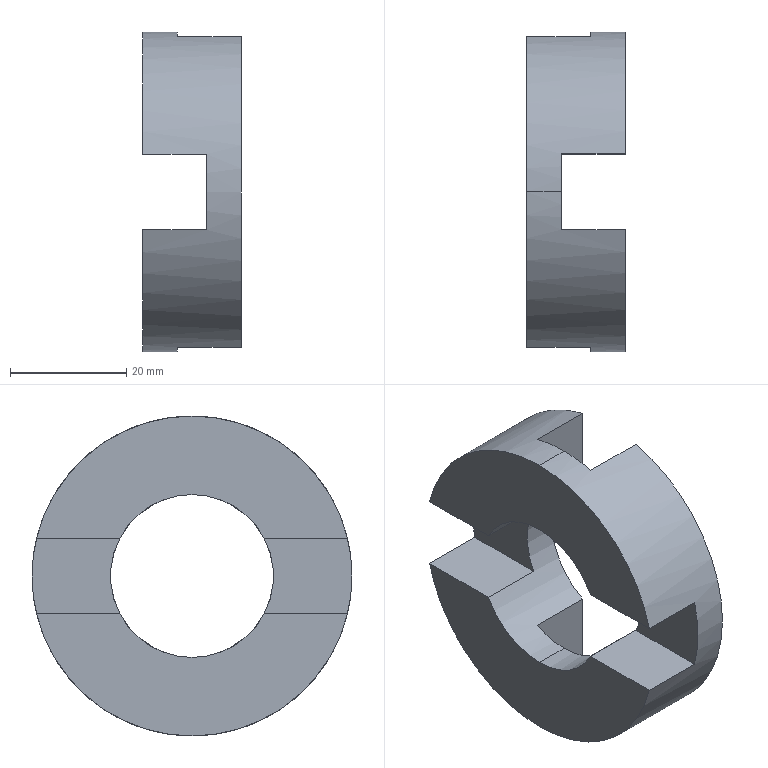Part | STEP file | 0229_Z_MFJC55-20-22_1 | 1 solid | 20 faces | box 17 x 55 x 55 mm | volume 22049 mm3 | plane 16 | cylinder 4 | commonest cylinder face diameters 28 x2 55 x2